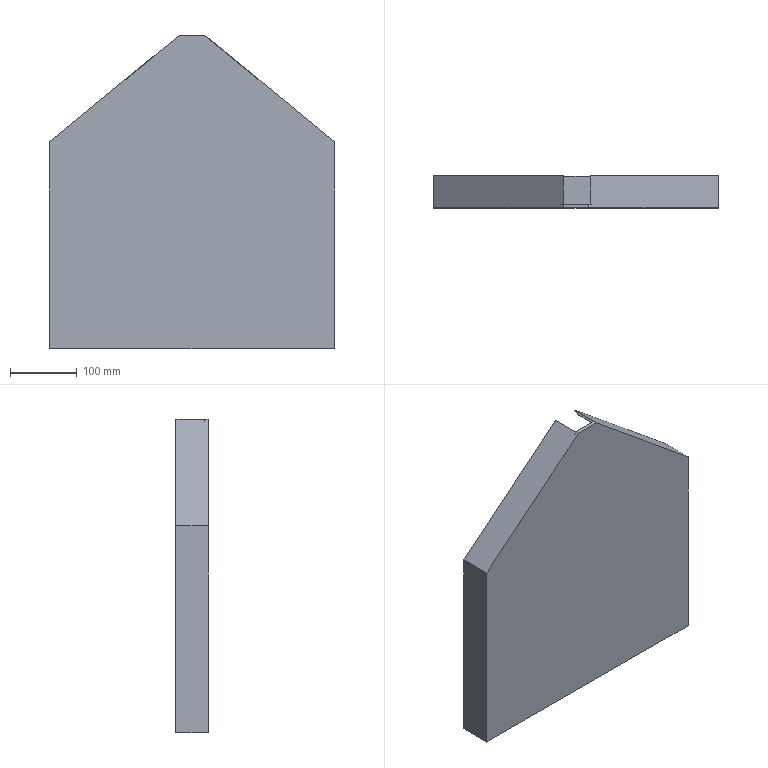Part | SolidWorks | features Cut 1, Extrusion 1, Shell 1 | 1 solid | 17 faces | box 425.348 x 48 x 468.238 mm | volume 1599795 mm3 | plane 17
STEP:
#1=CARTESIAN_POINT('',(-19.746,-48.,361.423));
#2=VERTEX_POINT('',#1);
#3=CARTESIAN_POINT('',(-19.746,-43.,361.423));
#4=VERTEX_POINT('',#3);
#5=CARTESIAN_POINT('',(-19.746,-48.,361.423));
#6=DIRECTION('',(0.,1.,0.));
#7=VECTOR('',#6,1000.);
#8=LINE('',#5,#7);
#9=EDGE_CURVE('',#2,#4,#8,.T.);
#10=ORIENTED_EDGE('',*,*,#9,.T.);
#11=CARTESIAN_POINT('',(-57.81,-43.,361.423));
#12=VERTEX_POINT('',#11);
#13=CARTESIAN_POINT('',(-57.81,-43.,361.423));
#14=DIRECTION('',(-1.,0.,0.));
#15=VECTOR('',#14,1000.);
#16=LINE('',#13,#15);
#17=EDGE_CURVE('',#4,#12,#16,.T.);
#18=ORIENTED_EDGE('',*,*,#17,.T.);
#19=CARTESIAN_POINT('',(-57.81,-48.,361.423));
#20=VERTEX_POINT('',#19);
#21=CARTESIAN_POINT('',(-57.81,-48.,361.423));
#22=DIRECTION('',(0.,1.,0.));
#23=VECTOR('',#22,1000.);
#24=LINE('',#21,#23);
#25=EDGE_CURVE('',#20,#12,#24,.T.);
#26=ORIENTED_EDGE('',*,*,#25,.F.);
#27=CARTESIAN_POINT('',(-57.81,-48.,361.423));
#28=DIRECTION('',(1.,0.,0.));
#29=VECTOR('',#28,1000.);
#30=LINE('',#27,#29);
#31=EDGE_CURVE('',#20,#2,#30,.T.);
#32=ORIENTED_EDGE('',*,*,#31,.T.);
#33=EDGE_LOOP('',(#10,#18,#26,#32));
#34=FACE_OUTER_BOUND('',#33,.T.);
#35=CARTESIAN_POINT('',(-57.81,-48.,361.423));
#36=DIRECTION('',(0.,0.,1.));
#37=DIRECTION('',(1.,0.,0.));
#38=AXIS2_PLACEMENT_3D('',#35,#36,#37);
#39=PLANE('',#38);
#40=ADVANCED_FACE('',(#34),#39,.T.);
#41=CARTESIAN_POINT('',(-67.862,0.,346.423));
#42=VERTEX_POINT('',#41);
#43=CARTESIAN_POINT('',(-58.065,0.,361.213));
#44=VERTEX_POINT('',#43);
#45=CARTESIAN_POINT('',(-56.918,0.,362.944));
#46=DIRECTION('',(0.5522,0.,0.8337));
#47=VECTOR('',#46,1000.);
#48=LINE('',#45,#47);
#49=EDGE_CURVE('',#42,#44,#48,.T.);
#50=ORIENTED_EDGE('',*,*,#49,.F.);
#51=CARTESIAN_POINT('',(-68.19,0.,346.423));
#52=VERTEX_POINT('',#51);
#53=CARTESIAN_POINT('',(0.,0.,346.423));
#54=DIRECTION('',(1.,0.,0.));
#55=VECTOR('',#54,1000.);
#56=LINE('',#53,#55);
#57=EDGE_CURVE('',#52,#42,#56,.T.);
#58=ORIENTED_EDGE('',*,*,#57,.F.);
#59=CARTESIAN_POINT('',(-236.451,0.,208.175));
#60=VERTEX_POINT('',#59);
#61=CARTESIAN_POINT('',(-197.402,0.,240.259));
#62=DIRECTION('',(-0.7727,0.,-0.6348));
#63=VECTOR('',#62,1000.);
#64=LINE('',#61,#63);
#65=EDGE_CURVE('',#52,#60,#64,.T.);
#66=ORIENTED_EDGE('',*,*,#65,.T.);
#67=CARTESIAN_POINT('',(-236.451,0.,-91.815));
#68=VERTEX_POINT('',#67);
#69=CARTESIAN_POINT('',(-236.451,0.,0.));
#70=DIRECTION('',(0.,0.,-1.));
#71=VECTOR('',#70,1000.);
#72=LINE('',#69,#71);
#73=EDGE_CURVE('',#60,#68,#72,.T.);
#74=ORIENTED_EDGE('',*,*,#73,.T.);
#75=CARTESIAN_POINT('',(158.896,0.,-91.815));
#76=VERTEX_POINT('',#75);
#77=CARTESIAN_POINT('',(0.,0.,-91.815));
#78=DIRECTION('',(1.,0.,0.));
#79=VECTOR('',#78,1000.);
#80=LINE('',#77,#79);
#81=EDGE_CURVE('',#68,#76,#80,.T.);
#82=ORIENTED_EDGE('',*,*,#81,.T.);
#83=CARTESIAN_POINT('',(158.896,0.,208.175));
#84=VERTEX_POINT('',#83);
#85=CARTESIAN_POINT('',(158.896,0.,0.));
#86=DIRECTION('',(0.,0.,1.));
#87=VECTOR('',#86,1000.);
#88=LINE('',#85,#87);
#89=EDGE_CURVE('',#76,#84,#88,.T.);
#90=ORIENTED_EDGE('',*,*,#89,.T.);
#91=CARTESIAN_POINT('',(-9.082,0.,346.191));
#92=VERTEX_POINT('',#91);
#93=CARTESIAN_POINT('',(166.147,0.,202.218));
#94=DIRECTION('',(-0.7727,0.,0.6348));
#95=VECTOR('',#94,1000.);
#96=LINE('',#93,#95);
#97=EDGE_CURVE('',#84,#92,#96,.T.);
#98=ORIENTED_EDGE('',*,*,#97,.T.);
#99=CARTESIAN_POINT('',(-17.753,0.,359.786));
#100=VERTEX_POINT('',#99);
#101=CARTESIAN_POINT('',(-19.767,0.,362.944));
#102=DIRECTION('',(0.5377,0.,-0.8431));
#103=VECTOR('',#102,1000.);
#104=LINE('',#101,#103);
#105=EDGE_CURVE('',#100,#92,#104,.T.);
#106=ORIENTED_EDGE('',*,*,#105,.F.);
#107=CARTESIAN_POINT('',(173.896,0.,202.322));
#108=VERTEX_POINT('',#107);
#109=CARTESIAN_POINT('',(173.896,0.,202.322));
#110=DIRECTION('',(-0.7727,0.,0.6348));
#111=VECTOR('',#110,1000.);
#112=LINE('',#109,#111);
#113=EDGE_CURVE('',#108,#100,#112,.T.);
#114=ORIENTED_EDGE('',*,*,#113,.F.);
#115=CARTESIAN_POINT('',(173.896,0.,-106.815));
#116=VERTEX_POINT('',#115);
#117=CARTESIAN_POINT('',(173.896,0.,-106.815));
#118=DIRECTION('',(0.,0.,1.));
#119=VECTOR('',#118,1000.);
#120=LINE('',#117,#119);
#121=EDGE_CURVE('',#116,#108,#120,.T.);
#122=ORIENTED_EDGE('',*,*,#121,.F.);
#123=CARTESIAN_POINT('',(-251.451,0.,-106.815));
#124=VERTEX_POINT('',#123);
#125=CARTESIAN_POINT('',(-251.451,0.,-106.815));
#126=DIRECTION('',(1.,0.,0.));
#127=VECTOR('',#126,1000.);
#128=LINE('',#125,#127);
#129=EDGE_CURVE('',#124,#116,#128,.T.);
#130=ORIENTED_EDGE('',*,*,#129,.F.);
#131=CARTESIAN_POINT('',(-251.451,0.,202.322));
#132=VERTEX_POINT('',#131);
#133=CARTESIAN_POINT('',(-251.451,0.,202.322));
#134=DIRECTION('',(0.,0.,-1.));
#135=VECTOR('',#134,1000.);
#136=LINE('',#133,#135);
#137=EDGE_CURVE('',#132,#124,#136,.T.);
#138=ORIENTED_EDGE('',*,*,#137,.F.);
#139=CARTESIAN_POINT('',(-57.81,0.,361.423));
#140=DIRECTION('',(-0.7727,0.,-0.6348));
#141=VECTOR('',#140,1000.);
#142=LINE('',#139,#141);
#143=EDGE_CURVE('',#44,#132,#142,.T.);
#144=ORIENTED_EDGE('',*,*,#143,.F.);
#145=EDGE_LOOP('',(#50,#58,#66,#74,#82,#90,#98,#106,#114,#122,#130,#138,#144));
#146=FACE_OUTER_BOUND('',#145,.T.);
#147=CARTESIAN_POINT('',(0.,0.,0.));
#148=DIRECTION('',(0.,1.,0.));
#149=DIRECTION('',(0.,0.,1.));
#150=AXIS2_PLACEMENT_3D('',#147,#148,#149);
#151=PLANE('',#150);
#152=ADVANCED_FACE('',(#146),#151,.T.);
#153=CARTESIAN_POINT('',(-58.065,-43.,361.213));
#154=VERTEX_POINT('',#153);
#155=CARTESIAN_POINT('',(-57.81,-43.,361.423));
#156=DIRECTION('',(0.7727,0.,0.6348));
#157=VECTOR('',#156,1000.);
#158=LINE('',#155,#157);
#159=EDGE_CURVE('',#154,#12,#158,.T.);
#160=ORIENTED_EDGE('',*,*,#159,.F.);
#161=CARTESIAN_POINT('',(-58.065,-48.,361.213));
#162=DIRECTION('',(0.,1.,0.));
#163=VECTOR('',#162,1000.);
#164=LINE('',#161,#163);
#165=EDGE_CURVE('',#154,#44,#164,.T.);
#166=ORIENTED_EDGE('',*,*,#165,.T.);
#167=ORIENTED_EDGE('',*,*,#143,.T.);
#168=CARTESIAN_POINT('',(-251.451,-48.,202.322));
#169=VERTEX_POINT('',#168);
#170=CARTESIAN_POINT('',(-251.451,-48.,202.322));
#171=DIRECTION('',(0.,1.,0.));
#172=VECTOR('',#171,1000.);
#173=LINE('',#170,#172);
#174=EDGE_CURVE('',#169,#132,#173,.T.);
#175=ORIENTED_EDGE('',*,*,#174,.F.);
#176=CARTESIAN_POINT('',(-57.81,-48.,361.423));
#177=DIRECTION('',(-0.7727,0.,-0.6348));
#178=VECTOR('',#177,1000.);
#179=LINE('',#176,#178);
#180=EDGE_CURVE('',#20,#169,#179,.T.);
#181=ORIENTED_EDGE('',*,*,#180,.F.);
#182=ORIENTED_EDGE('',*,*,#25,.T.);
#183=EDGE_LOOP('',(#160,#166,#167,#175,#181,#182));
#184=FACE_OUTER_BOUND('',#183,.T.);
#185=CARTESIAN_POINT('',(-57.81,-48.,361.423));
#186=DIRECTION('',(0.6348,0.,-0.7727));
#187=DIRECTION('',(-0.7727,0.,-0.6348));
#188=AXIS2_PLACEMENT_3D('',#185,#186,#187);
#189=PLANE('',#188);
#190=ADVANCED_FACE('',(#184),#189,.F.);
#191=ORIENTED_EDGE('',*,*,#137,.T.);
#192=CARTESIAN_POINT('',(-251.451,-48.,-106.815));
#193=VERTEX_POINT('',#192);
#194=CARTESIAN_POINT('',(-251.451,-48.,-106.815));
#195=DIRECTION('',(0.,1.,0.));
#196=VECTOR('',#195,1000.);
#197=LINE('',#194,#196);
#198=EDGE_CURVE('',#193,#124,#197,.T.);
#199=ORIENTED_EDGE('',*,*,#198,.F.);
#200=CARTESIAN_POINT('',(-251.451,-48.,202.322));
#201=DIRECTION('',(0.,0.,-1.));
#202=VECTOR('',#201,1000.);
#203=LINE('',#200,#202);
#204=EDGE_CURVE('',#169,#193,#203,.T.);
#205=ORIENTED_EDGE('',*,*,#204,.F.);
#206=ORIENTED_EDGE('',*,*,#174,.T.);
#207=EDGE_LOOP('',(#191,#199,#205,#206));
#208=FACE_OUTER_BOUND('',#207,.T.);
#209=CARTESIAN_POINT('',(-251.451,-48.,202.322));
#210=DIRECTION('',(1.,0.,0.));
#211=DIRECTION('',(0.,0.,-1.));
#212=AXIS2_PLACEMENT_3D('',#209,#210,#211);
#213=PLANE('',#212);
#214=ADVANCED_FACE('',(#208),#213,.F.);
#215=ORIENTED_EDGE('',*,*,#129,.T.);
#216=CARTESIAN_POINT('',(173.896,-48.,-106.815));
#217=VERTEX_POINT('',#216);
#218=CARTESIAN_POINT('',(173.896,-48.,-106.815));
#219=DIRECTION('',(0.,1.,0.));
#220=VECTOR('',#219,1000.);
#221=LINE('',#218,#220);
#222=EDGE_CURVE('',#217,#116,#221,.T.);
#223=ORIENTED_EDGE('',*,*,#222,.F.);
#224=CARTESIAN_POINT('',(-251.451,-48.,-106.815));
#225=DIRECTION('',(1.,0.,0.));
#226=VECTOR('',#225,1000.);
#227=LINE('',#224,#226);
#228=EDGE_CURVE('',#193,#217,#227,.T.);
#229=ORIENTED_EDGE('',*,*,#228,.F.);
#230=ORIENTED_EDGE('',*,*,#198,.T.);
#231=EDGE_LOOP('',(#215,#223,#229,#230));
#232=FACE_OUTER_BOUND('',#231,.T.);
#233=CARTESIAN_POINT('',(-251.451,-48.,-106.815));
#234=DIRECTION('',(0.,0.,1.));
#235=DIRECTION('',(1.,0.,0.));
#236=AXIS2_PLACEMENT_3D('',#233,#234,#235);
#237=PLANE('',#236);
#238=ADVANCED_FACE('',(#232),#237,.F.);
#239=ORIENTED_EDGE('',*,*,#121,.T.);
#240=CARTESIAN_POINT('',(173.896,-48.,202.322));
#241=VERTEX_POINT('',#240);
#242=CARTESIAN_POINT('',(173.896,-48.,202.322));
#243=DIRECTION('',(0.,1.,0.));
#244=VECTOR('',#243,1000.);
#245=LINE('',#242,#244);
#246=EDGE_CURVE('',#241,#108,#245,.T.);
#247=ORIENTED_EDGE('',*,*,#246,.F.);
#248=CARTESIAN_POINT('',(173.896,-48.,-106.815));
#249=DIRECTION('',(0.,0.,1.));
#250=VECTOR('',#249,1000.);
#251=LINE('',#248,#250);
#252=EDGE_CURVE('',#217,#241,#251,.T.);
#253=ORIENTED_EDGE('',*,*,#252,.F.);
#254=ORIENTED_EDGE('',*,*,#222,.T.);
#255=EDGE_LOOP('',(#239,#247,#253,#254));
#256=FACE_OUTER_BOUND('',#255,.T.);
#257=CARTESIAN_POINT('',(173.896,-48.,-106.815));
#258=DIRECTION('',(-1.,0.,0.));
#259=DIRECTION('',(0.,0.,1.));
#260=AXIS2_PLACEMENT_3D('',#257,#258,#259);
#261=PLANE('',#260);
#262=ADVANCED_FACE('',(#256),#261,.F.);
#263=ORIENTED_EDGE('',*,*,#113,.T.);
#264=CARTESIAN_POINT('',(-17.753,-43.,359.786));
#265=VERTEX_POINT('',#264);
#266=CARTESIAN_POINT('',(-17.753,-48.,359.786));
#267=DIRECTION('',(0.,-1.,0.));
#268=VECTOR('',#267,1000.);
#269=LINE('',#266,#268);
#270=EDGE_CURVE('',#100,#265,#269,.T.);
#271=ORIENTED_EDGE('',*,*,#270,.T.);
#272=CARTESIAN_POINT('',(173.896,-43.,202.322));
#273=DIRECTION('',(0.7727,0.,-0.6348));
#274=VECTOR('',#273,1000.);
#275=LINE('',#272,#274);
#276=EDGE_CURVE('',#4,#265,#275,.T.);
#277=ORIENTED_EDGE('',*,*,#276,.F.);
#278=ORIENTED_EDGE('',*,*,#9,.F.);
#279=CARTESIAN_POINT('',(173.896,-48.,202.322));
#280=DIRECTION('',(-0.7727,0.,0.6348));
#281=VECTOR('',#280,1000.);
#282=LINE('',#279,#281);
#283=EDGE_CURVE('',#241,#2,#282,.T.);
#284=ORIENTED_EDGE('',*,*,#283,.F.);
#285=ORIENTED_EDGE('',*,*,#246,.T.);
#286=EDGE_LOOP('',(#263,#271,#277,#278,#284,#285));
#287=FACE_OUTER_BOUND('',#286,.T.);
#288=CARTESIAN_POINT('',(173.896,-48.,202.322));
#289=DIRECTION('',(-0.6348,0.,-0.7727));
#290=DIRECTION('',(-0.7727,0.,0.6348));
#291=AXIS2_PLACEMENT_3D('',#288,#289,#290);
#292=PLANE('',#291);
#293=ADVANCED_FACE('',(#287),#292,.F.);
#294=ORIENTED_EDGE('',*,*,#180,.T.);
#295=ORIENTED_EDGE('',*,*,#204,.T.);
#296=ORIENTED_EDGE('',*,*,#228,.T.);
#297=ORIENTED_EDGE('',*,*,#252,.T.);
#298=ORIENTED_EDGE('',*,*,#283,.T.);
#299=ORIENTED_EDGE('',*,*,#31,.F.);
#300=EDGE_LOOP('',(#294,#295,#296,#297,#298,#299));
#301=FACE_OUTER_BOUND('',#300,.T.);
#302=CARTESIAN_POINT('',(0.,-48.,0.));
#303=DIRECTION('',(0.,1.,0.));
#304=DIRECTION('',(0.,0.,1.));
#305=AXIS2_PLACEMENT_3D('',#302,#303,#304);
#306=PLANE('',#305);
#307=ADVANCED_FACE('',(#301),#306,.F.);
#308=ORIENTED_EDGE('',*,*,#65,.F.);
#309=CARTESIAN_POINT('',(-68.19,-43.,346.423));
#310=VERTEX_POINT('',#309);
#311=CARTESIAN_POINT('',(-68.19,-48.,346.423));
#312=DIRECTION('',(0.,1.,0.));
#313=VECTOR('',#312,1000.);
#314=LINE('',#311,#313);
#315=EDGE_CURVE('',#310,#52,#314,.T.);
#316=ORIENTED_EDGE('',*,*,#315,.F.);
#317=CARTESIAN_POINT('',(-236.451,-43.,208.175));
#318=VERTEX_POINT('',#317);
#319=CARTESIAN_POINT('',(-197.402,-43.,240.259));
#320=DIRECTION('',(-0.7727,0.,-0.6348));
#321=VECTOR('',#320,1000.);
#322=LINE('',#319,#321);
#323=EDGE_CURVE('',#310,#318,#322,.T.);
#324=ORIENTED_EDGE('',*,*,#323,.T.);
#325=CARTESIAN_POINT('',(-236.451,-48.,208.175));
#326=DIRECTION('',(0.,1.,0.));
#327=VECTOR('',#326,1000.);
#328=LINE('',#325,#327);
#329=EDGE_CURVE('',#318,#60,#328,.T.);
#330=ORIENTED_EDGE('',*,*,#329,.T.);
#331=EDGE_LOOP('',(#308,#316,#324,#330));
#332=FACE_OUTER_BOUND('',#331,.T.);
#333=CARTESIAN_POINT('',(-54.635,-48.,357.56));
#334=DIRECTION('',(0.6348,0.,-0.7727));
#335=DIRECTION('',(-0.7727,0.,-0.6348));
#336=AXIS2_PLACEMENT_3D('',#333,#334,#335);
#337=PLANE('',#336);
#338=ADVANCED_FACE('',(#332),#337,.T.);
#339=ORIENTED_EDGE('',*,*,#73,.F.);
#340=ORIENTED_EDGE('',*,*,#329,.F.);
#341=CARTESIAN_POINT('',(-236.451,-43.,-91.815));
#342=VERTEX_POINT('',#341);
#343=CARTESIAN_POINT('',(-236.451,-43.,0.));
#344=DIRECTION('',(0.,0.,-1.));
#345=VECTOR('',#344,1000.);
#346=LINE('',#343,#345);
#347=EDGE_CURVE('',#318,#342,#346,.T.);
#348=ORIENTED_EDGE('',*,*,#347,.T.);
#349=CARTESIAN_POINT('',(-236.451,-48.,-91.815));
#350=DIRECTION('',(0.,1.,0.));
#351=VECTOR('',#350,1000.);
#352=LINE('',#349,#351);
#353=EDGE_CURVE('',#342,#68,#352,.T.);
#354=ORIENTED_EDGE('',*,*,#353,.T.);
#355=EDGE_LOOP('',(#339,#340,#348,#354));
#356=FACE_OUTER_BOUND('',#355,.T.);
#357=CARTESIAN_POINT('',(-236.451,-48.,202.322));
#358=DIRECTION('',(1.,0.,0.));
#359=DIRECTION('',(0.,0.,-1.));
#360=AXIS2_PLACEMENT_3D('',#357,#358,#359);
#361=PLANE('',#360);
#362=ADVANCED_FACE('',(#356),#361,.T.);
#363=ORIENTED_EDGE('',*,*,#81,.F.);
#364=ORIENTED_EDGE('',*,*,#353,.F.);
#365=CARTESIAN_POINT('',(158.896,-43.,-91.815));
#366=VERTEX_POINT('',#365);
#367=CARTESIAN_POINT('',(0.,-43.,-91.815));
#368=DIRECTION('',(1.,0.,0.));
#369=VECTOR('',#368,1000.);
#370=LINE('',#367,#369);
#371=EDGE_CURVE('',#342,#366,#370,.T.);
#372=ORIENTED_EDGE('',*,*,#371,.T.);
#373=CARTESIAN_POINT('',(158.896,-48.,-91.815));
#374=DIRECTION('',(0.,1.,0.));
#375=VECTOR('',#374,1000.);
#376=LINE('',#373,#375);
#377=EDGE_CURVE('',#366,#76,#376,.T.);
#378=ORIENTED_EDGE('',*,*,#377,.T.);
#379=EDGE_LOOP('',(#363,#364,#372,#378));
#380=FACE_OUTER_BOUND('',#379,.T.);
#381=CARTESIAN_POINT('',(-251.451,-48.,-91.815));
#382=DIRECTION('',(0.,0.,1.));
#383=DIRECTION('',(1.,0.,0.));
#384=AXIS2_PLACEMENT_3D('',#381,#382,#383);
#385=PLANE('',#384);
#386=ADVANCED_FACE('',(#380),#385,.T.);
#387=ORIENTED_EDGE('',*,*,#89,.F.);
#388=ORIENTED_EDGE('',*,*,#377,.F.);
#389=CARTESIAN_POINT('',(158.896,-43.,208.175));
#390=VERTEX_POINT('',#389);
#391=CARTESIAN_POINT('',(158.896,-43.,0.));
#392=DIRECTION('',(0.,0.,1.));
#393=VECTOR('',#392,1000.);
#394=LINE('',#391,#393);
#395=EDGE_CURVE('',#366,#390,#394,.T.);
#396=ORIENTED_EDGE('',*,*,#395,.T.);
#397=CARTESIAN_POINT('',(158.896,-48.,208.175));
#398=DIRECTION('',(0.,1.,0.));
#399=VECTOR('',#398,1000.);
#400=LINE('',#397,#399);
#401=EDGE_CURVE('',#390,#84,#400,.T.);
#402=ORIENTED_EDGE('',*,*,#401,.T.);
#403=EDGE_LOOP('',(#387,#388,#396,#402));
#404=FACE_OUTER_BOUND('',#403,.T.);
#405=CARTESIAN_POINT('',(158.896,-48.,-106.815));
#406=DIRECTION('',(-1.,0.,0.));
#407=DIRECTION('',(0.,0.,1.));
#408=AXIS2_PLACEMENT_3D('',#405,#406,#407);
#409=PLANE('',#408);
#410=ADVANCED_FACE('',(#404),#409,.T.);
#411=CARTESIAN_POINT('',(-9.082,-43.,346.191));
#412=VERTEX_POINT('',#411);
#413=CARTESIAN_POINT('',(-9.082,-48.,346.191));
#414=DIRECTION('',(0.,-1.,0.));
#415=VECTOR('',#414,1000.);
#416=LINE('',#413,#415);
#417=EDGE_CURVE('',#92,#412,#416,.T.);
#418=ORIENTED_EDGE('',*,*,#417,.F.);
#419=ORIENTED_EDGE('',*,*,#97,.F.);
#420=ORIENTED_EDGE('',*,*,#401,.F.);
#421=CARTESIAN_POINT('',(166.147,-43.,202.218));
#422=DIRECTION('',(-0.7727,0.,0.6348));
#423=VECTOR('',#422,1000.);
#424=LINE('',#421,#423);
#425=EDGE_CURVE('',#390,#412,#424,.T.);
#426=ORIENTED_EDGE('',*,*,#425,.T.);
#427=EDGE_LOOP('',(#418,#419,#420,#426));
#428=FACE_OUTER_BOUND('',#427,.T.);
#429=CARTESIAN_POINT('',(170.722,-48.,198.459));
#430=DIRECTION('',(-0.6348,0.,-0.7727));
#431=DIRECTION('',(-0.7727,0.,0.6348));
#432=AXIS2_PLACEMENT_3D('',#429,#430,#431);
#433=PLANE('',#432);
#434=ADVANCED_FACE('',(#428),#433,.T.);
#435=ORIENTED_EDGE('',*,*,#57,.T.);
#436=CARTESIAN_POINT('',(-67.862,-43.,346.423));
#437=VERTEX_POINT('',#436);
#438=CARTESIAN_POINT('',(-67.862,-48.,346.423));
#439=DIRECTION('',(0.,-1.,0.));
#440=VECTOR('',#439,1000.);
#441=LINE('',#438,#440);
#442=EDGE_CURVE('',#42,#437,#441,.T.);
#443=ORIENTED_EDGE('',*,*,#442,.T.);
#444=CARTESIAN_POINT('',(0.,-43.,346.423));
#445=DIRECTION('',(1.,0.,0.));
#446=VECTOR('',#445,1000.);
#447=LINE('',#444,#446);
#448=EDGE_CURVE('',#310,#437,#447,.T.);
#449=ORIENTED_EDGE('',*,*,#448,.F.);
#450=ORIENTED_EDGE('',*,*,#315,.T.);
#451=EDGE_LOOP('',(#435,#443,#449,#450));
#452=FACE_OUTER_BOUND('',#451,.T.);
#453=CARTESIAN_POINT('',(-57.81,-48.,346.423));
#454=DIRECTION('',(0.,0.,1.));
#455=DIRECTION('',(1.,0.,0.));
#456=AXIS2_PLACEMENT_3D('',#453,#454,#455);
#457=PLANE('',#456);
#458=ADVANCED_FACE('',(#452),#457,.F.);
#459=ORIENTED_EDGE('',*,*,#448,.T.);
#460=CARTESIAN_POINT('',(-56.918,-43.,362.944));
#461=DIRECTION('',(0.5522,0.,0.8337));
#462=VECTOR('',#461,1000.);
#463=LINE('',#460,#462);
#464=EDGE_CURVE('',#437,#154,#463,.T.);
#465=ORIENTED_EDGE('',*,*,#464,.T.);
#466=ORIENTED_EDGE('',*,*,#159,.T.);
#467=ORIENTED_EDGE('',*,*,#17,.F.);
#468=ORIENTED_EDGE('',*,*,#276,.T.);
#469=CARTESIAN_POINT('',(-19.767,-43.,362.944));
#470=DIRECTION('',(0.5377,0.,-0.8431));
#471=VECTOR('',#470,1000.);
#472=LINE('',#469,#471);
#473=EDGE_CURVE('',#265,#412,#472,.T.);
#474=ORIENTED_EDGE('',*,*,#473,.T.);
#475=ORIENTED_EDGE('',*,*,#425,.F.);
#476=ORIENTED_EDGE('',*,*,#395,.F.);
#477=ORIENTED_EDGE('',*,*,#371,.F.);
#478=ORIENTED_EDGE('',*,*,#347,.F.);
#479=ORIENTED_EDGE('',*,*,#323,.F.);
#480=EDGE_LOOP('',(#459,#465,#466,#467,#468,#474,#475,#476,#477,#478,#479));
#481=FACE_OUTER_BOUND('',#480,.T.);
#482=CARTESIAN_POINT('',(0.,-43.,0.));
#483=DIRECTION('',(0.,1.,0.));
#484=DIRECTION('',(0.,0.,1.));
#485=AXIS2_PLACEMENT_3D('',#482,#483,#484);
#486=PLANE('',#485);
#487=ADVANCED_FACE('',(#481),#486,.T.);
#488=ORIENTED_EDGE('',*,*,#464,.F.);
#489=ORIENTED_EDGE('',*,*,#442,.F.);
#490=ORIENTED_EDGE('',*,*,#49,.T.);
#491=ORIENTED_EDGE('',*,*,#165,.F.);
#492=EDGE_LOOP('',(#488,#489,#490,#491));
#493=FACE_OUTER_BOUND('',#492,.T.);
#494=CARTESIAN_POINT('',(-56.918,-43.,362.944));
#495=DIRECTION('',(-0.8337,0.,0.5522));
#496=DIRECTION('',(0.5522,0.,0.8337));
#497=AXIS2_PLACEMENT_3D('',#494,#495,#496);
#498=PLANE('',#497);
#499=ADVANCED_FACE('',(#493),#498,.F.);
#500=ORIENTED_EDGE('',*,*,#105,.T.);
#501=ORIENTED_EDGE('',*,*,#417,.T.);
#502=ORIENTED_EDGE('',*,*,#473,.F.);
#503=ORIENTED_EDGE('',*,*,#270,.F.);
#504=EDGE_LOOP('',(#500,#501,#502,#503));
#505=FACE_OUTER_BOUND('',#504,.T.);
#506=CARTESIAN_POINT('',(-19.767,-43.,362.944));
#507=DIRECTION('',(0.8431,0.,0.5377));
#508=DIRECTION('',(0.5377,0.,-0.8431));
#509=AXIS2_PLACEMENT_3D('',#506,#507,#508);
#510=PLANE('',#509);
#511=ADVANCED_FACE('',(#505),#510,.F.);
#512=CLOSED_SHELL('',(#40,#152,#190,#214,#238,#262,#293,#307,#338,#362,#386,#410,#434,#458,#487,#499,#511));
#513=MANIFOLD_SOLID_BREP('',#512);
#514=CARTESIAN_POINT('',(0.,0.,0.));
#515=DIRECTION('',(0.,0.,1.));
#516=DIRECTION('',(1.,0.,0.));
#517=AXIS2_PLACEMENT_3D('',#514,#515,#516);
#518=(LENGTH_UNIT()NAMED_UNIT(*)SI_UNIT(.MILLI.,.METRE.));
#519=UNCERTAINTY_MEASURE_WITH_UNIT(LENGTH_MEASURE(0.00001),#518,'','');
#520=(NAMED_UNIT(*)PLANE_ANGLE_UNIT()SI_UNIT($,.RADIAN.));
#521=(NAMED_UNIT(*)SI_UNIT($,.STERADIAN.)SOLID_ANGLE_UNIT());
#522=(GEOMETRIC_REPRESENTATION_CONTEXT(3)GLOBAL_UNCERTAINTY_ASSIGNED_CONTEXT((#519))GLOBAL_UNIT_ASSIGNED_CONTEXT((#518,#520,#521))REPRESENTATION_CONTEXT('',''));
#523=ADVANCED_BREP_SHAPE_REPRESENTATION('',(#513,#517),#522);